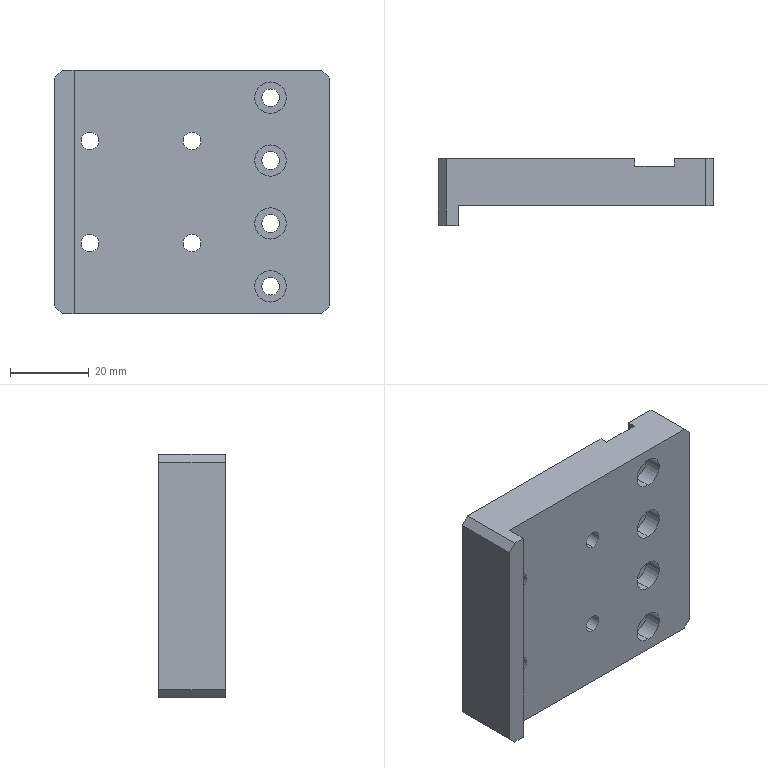Part | SolidWorks | features BaseBody 1 | 1 solid | 56 faces | box 70 x 17 x 62 mm | volume 49610 mm3 | cylinder 32 | plane 24 | commonest cylinder face diameters 4.5 x16 8 x16